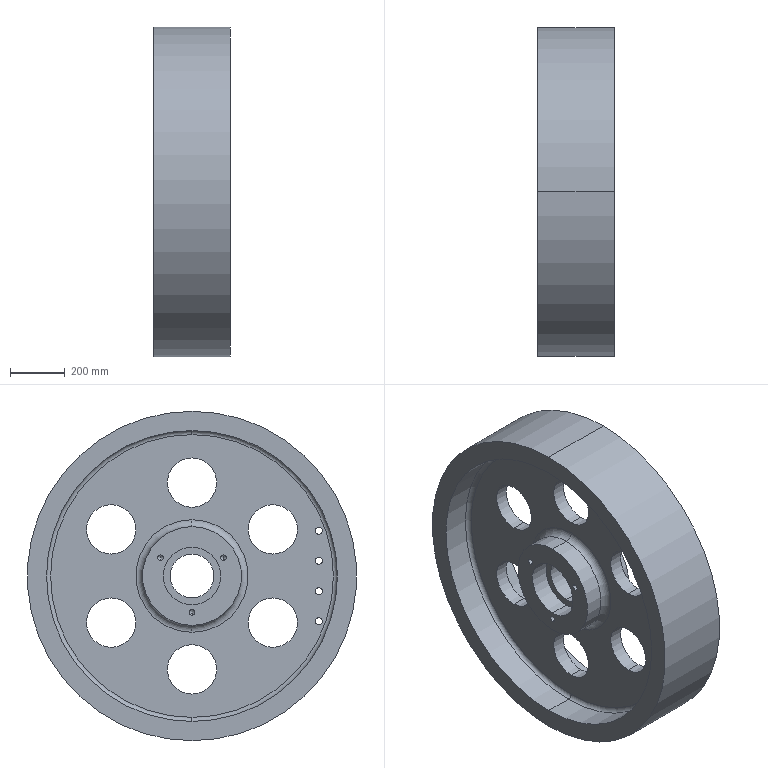Part | SolidWorks | features CirPattern 2, ICE 2, 3DProfileFeature 1, HoleWzd 1, Revolution 1 | 1 solid | 61 faces | box 280 x 1200 x 1200 mm | volume 117077142 mm3 | cylinder 40 | torus 8 | plane 7 | cone 6 | commonest cylinder face diameters 180 x12 25 x8 21 x6 1060 x4 160 x2 210 x2